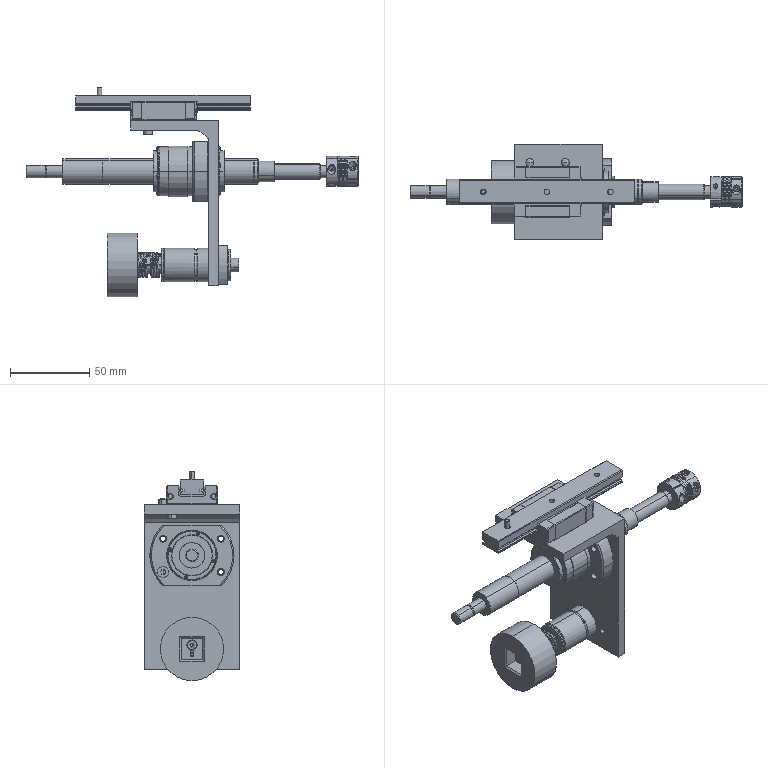Part | SolidWorks | features AEMSimFeature 1, CompositeCurve 1 | 27 solids | 1126 faces | box 209.2 x 60 x 132 mm | volume 185380 mm3 | plane 588 | cylinder 364 | cone 155 | spline 9 | sphere 6 | torus 4 | commonest cylinder face diameters 0.4 x30 2.5 x26 3.5 x22 4.5 x20 3.4 x18 2.24 x16